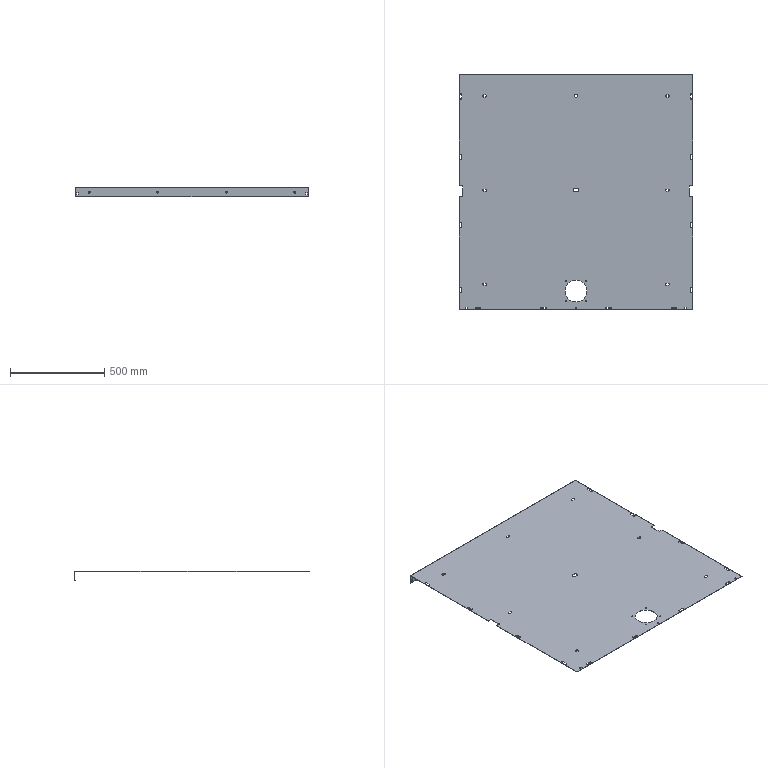Part | 1 solid | 172 faces | box 1240 x 1250 x 49.5 mm | volume 2395440 mm3 | plane 90 | cylinder 82 | commonest cylinder face diameters 10 x30 11 x21 5.9 x8 10.5 x8 6 x4 20 x3